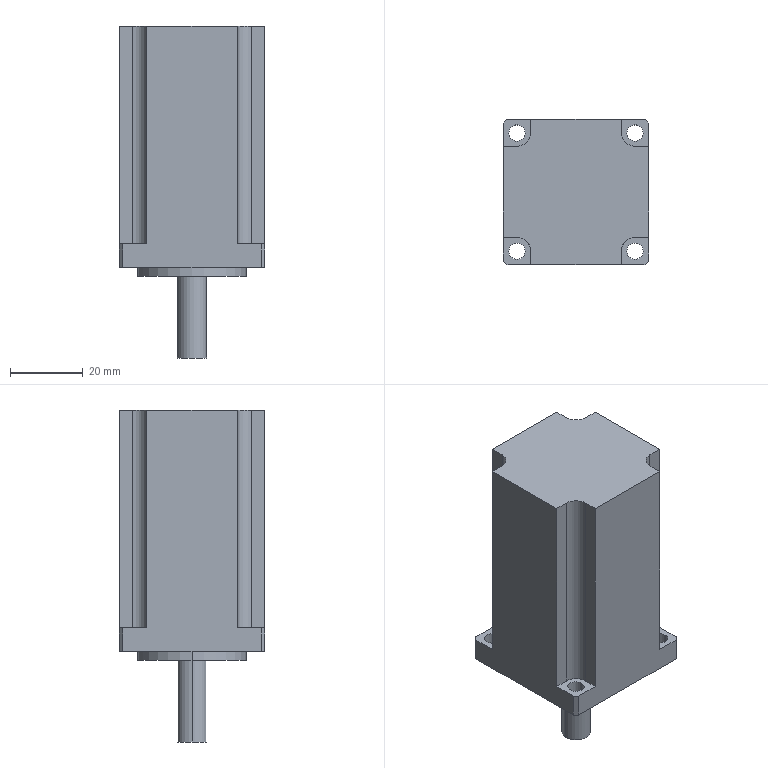Part | Creo | features CURVE 4, DATUM PLANE 3, PROTRUSION 3, CHAMFER 1, COORDINATE SYSTEM 1, CUT 1 | 1 solid | 40 faces | box 40 x 40 x 91.4 mm | volume 96010 mm3 | plane 24 | cylinder 16 | commonest cylinder face diameters 4.5 x8 7.48 x4 8 x2 30 x2
STEP:
#1=CARTESIAN_POINT('',(0.,0.,0.));
#2=DIRECTION('',(0.,0.,1.));
#3=DIRECTION('',(1.,0.,0.));
#4=AXIS2_PLACEMENT_3D('',#1,#2,#3);
#5=CARTESIAN_POINT('',(19.,20.,0.));
#6=VERTEX_POINT('',#5);
#7=CARTESIAN_POINT('',(20.,19.,0.));
#8=VERTEX_POINT('',#7);
#9=CARTESIAN_POINT('',(19.,20.,0.));
#10=DIRECTION('',(0.7071,-0.7071,0.));
#11=VECTOR('',#10,1.414);
#12=LINE('',#9,#11);
#13=EDGE_CURVE('',#6,#8,#12,.T.);
#14=ORIENTED_EDGE('',*,*,#13,.F.);
#15=CARTESIAN_POINT('',(-19.,20.,0.));
#16=VERTEX_POINT('',#15);
#17=CARTESIAN_POINT('',(19.,20.,0.));
#18=DIRECTION('',(-1.,0.,0.));
#19=VECTOR('',#18,38.);
#20=LINE('',#17,#19);
#21=EDGE_CURVE('',#6,#16,#20,.T.);
#22=ORIENTED_EDGE('',*,*,#21,.T.);
#23=CARTESIAN_POINT('',(-20.,19.,0.));
#24=VERTEX_POINT('',#23);
#25=CARTESIAN_POINT('',(-20.,19.,0.));
#26=DIRECTION('',(0.7071,0.7071,0.));
#27=VECTOR('',#26,1.414);
#28=LINE('',#25,#27);
#29=EDGE_CURVE('',#24,#16,#28,.T.);
#30=ORIENTED_EDGE('',*,*,#29,.F.);
#31=CARTESIAN_POINT('',(-20.,-19.,0.));
#32=VERTEX_POINT('',#31);
#33=CARTESIAN_POINT('',(-20.,19.,0.));
#34=DIRECTION('',(0.,-1.,0.));
#35=VECTOR('',#34,38.);
#36=LINE('',#33,#35);
#37=EDGE_CURVE('',#24,#32,#36,.T.);
#38=ORIENTED_EDGE('',*,*,#37,.T.);
#39=CARTESIAN_POINT('',(-19.,-20.,0.));
#40=VERTEX_POINT('',#39);
#41=CARTESIAN_POINT('',(-19.,-20.,0.));
#42=DIRECTION('',(-0.7071,0.7071,0.));
#43=VECTOR('',#42,1.414);
#44=LINE('',#41,#43);
#45=EDGE_CURVE('',#40,#32,#44,.T.);
#46=ORIENTED_EDGE('',*,*,#45,.F.);
#47=CARTESIAN_POINT('',(19.,-20.,0.));
#48=VERTEX_POINT('',#47);
#49=CARTESIAN_POINT('',(-19.,-20.,0.));
#50=DIRECTION('',(1.,0.,0.));
#51=VECTOR('',#50,38.);
#52=LINE('',#49,#51);
#53=EDGE_CURVE('',#40,#48,#52,.T.);
#54=ORIENTED_EDGE('',*,*,#53,.T.);
#55=CARTESIAN_POINT('',(20.,-19.,0.));
#56=VERTEX_POINT('',#55);
#57=CARTESIAN_POINT('',(20.,-19.,0.));
#58=DIRECTION('',(-0.7071,-0.7071,0.));
#59=VECTOR('',#58,1.414);
#60=LINE('',#57,#59);
#61=EDGE_CURVE('',#56,#48,#60,.T.);
#62=ORIENTED_EDGE('',*,*,#61,.F.);
#63=CARTESIAN_POINT('',(20.,-19.,0.));
#64=DIRECTION('',(0.,1.,0.));
#65=VECTOR('',#64,38.);
#66=LINE('',#63,#65);
#67=EDGE_CURVE('',#56,#8,#66,.T.);
#68=ORIENTED_EDGE('',*,*,#67,.T.);
#69=EDGE_LOOP('',(#14,#22,#30,#38,#46,#54,#62,#68));
#70=FACE_OUTER_BOUND('',#69,.F.);
#71=CARTESIAN_POINT('',(-14.01,16.26,0.));
#72=VERTEX_POINT('',#71);
#73=CARTESIAN_POINT('',(-18.51,16.26,0.));
#74=VERTEX_POINT('',#73);
#75=CARTESIAN_POINT('',(-16.26,16.26,0.));
#76=DIRECTION('',(0.,0.,-1.));
#77=DIRECTION('',(1.,0.,0.));
#78=AXIS2_PLACEMENT_3D('',#75,#76,#77);
#79=CIRCLE('',#78,2.25);
#80=EDGE_CURVE('',#72,#74,#79,.T.);
#81=ORIENTED_EDGE('',*,*,#80,.T.);
#82=CARTESIAN_POINT('',(-16.26,16.26,0.));
#83=DIRECTION('',(0.,0.,-1.));
#84=DIRECTION('',(-1.,0.,0.));
#85=AXIS2_PLACEMENT_3D('',#82,#83,#84);
#86=CIRCLE('',#85,2.25);
#87=EDGE_CURVE('',#74,#72,#86,.T.);
#88=ORIENTED_EDGE('',*,*,#87,.T.);
#89=EDGE_LOOP('',(#81,#88));
#90=FACE_BOUND('',#89,.F.);
#91=CARTESIAN_POINT('',(-14.01,-16.26,0.));
#92=VERTEX_POINT('',#91);
#93=CARTESIAN_POINT('',(-18.51,-16.26,0.));
#94=VERTEX_POINT('',#93);
#95=CARTESIAN_POINT('',(-16.26,-16.26,0.));
#96=DIRECTION('',(0.,0.,-1.));
#97=DIRECTION('',(1.,0.,0.));
#98=AXIS2_PLACEMENT_3D('',#95,#96,#97);
#99=CIRCLE('',#98,2.25);
#100=EDGE_CURVE('',#92,#94,#99,.T.);
#101=ORIENTED_EDGE('',*,*,#100,.T.);
#102=CARTESIAN_POINT('',(-16.26,-16.26,0.));
#103=DIRECTION('',(0.,0.,-1.));
#104=DIRECTION('',(-1.,0.,0.));
#105=AXIS2_PLACEMENT_3D('',#102,#103,#104);
#106=CIRCLE('',#105,2.25);
#107=EDGE_CURVE('',#94,#92,#106,.T.);
#108=ORIENTED_EDGE('',*,*,#107,.T.);
#109=EDGE_LOOP('',(#101,#108));
#110=FACE_BOUND('',#109,.F.);
#111=CARTESIAN_POINT('',(18.51,-16.26,0.));
#112=VERTEX_POINT('',#111);
#113=CARTESIAN_POINT('',(14.01,-16.26,0.));
#114=VERTEX_POINT('',#113);
#115=CARTESIAN_POINT('',(16.26,-16.26,0.));
#116=DIRECTION('',(0.,0.,-1.));
#117=DIRECTION('',(1.,0.,0.));
#118=AXIS2_PLACEMENT_3D('',#115,#116,#117);
#119=CIRCLE('',#118,2.25);
#120=EDGE_CURVE('',#112,#114,#119,.T.);
#121=ORIENTED_EDGE('',*,*,#120,.T.);
#122=CARTESIAN_POINT('',(16.26,-16.26,0.));
#123=DIRECTION('',(0.,0.,-1.));
#124=DIRECTION('',(-1.,0.,0.));
#125=AXIS2_PLACEMENT_3D('',#122,#123,#124);
#126=CIRCLE('',#125,2.25);
#127=EDGE_CURVE('',#114,#112,#126,.T.);
#128=ORIENTED_EDGE('',*,*,#127,.T.);
#129=EDGE_LOOP('',(#121,#128));
#130=FACE_BOUND('',#129,.F.);
#131=CARTESIAN_POINT('',(18.51,16.26,0.));
#132=VERTEX_POINT('',#131);
#133=CARTESIAN_POINT('',(14.01,16.26,0.));
#134=VERTEX_POINT('',#133);
#135=CARTESIAN_POINT('',(16.26,16.26,0.));
#136=DIRECTION('',(0.,0.,-1.));
#137=DIRECTION('',(1.,0.,0.));
#138=AXIS2_PLACEMENT_3D('',#135,#136,#137);
#139=CIRCLE('',#138,2.25);
#140=EDGE_CURVE('',#132,#134,#139,.T.);
#141=ORIENTED_EDGE('',*,*,#140,.T.);
#142=CARTESIAN_POINT('',(16.26,16.26,0.));
#143=DIRECTION('',(0.,0.,-1.));
#144=DIRECTION('',(-1.,0.,0.));
#145=AXIS2_PLACEMENT_3D('',#142,#143,#144);
#146=CIRCLE('',#145,2.25);
#147=EDGE_CURVE('',#134,#132,#146,.T.);
#148=ORIENTED_EDGE('',*,*,#147,.T.);
#149=EDGE_LOOP('',(#141,#148));
#150=FACE_BOUND('',#149,.F.);
#151=CARTESIAN_POINT('',(-15.,0.,0.));
#152=VERTEX_POINT('',#151);
#153=CARTESIAN_POINT('',(15.,0.,0.));
#154=VERTEX_POINT('',#153);
#155=CARTESIAN_POINT('',(0.,0.,0.));
#156=DIRECTION('',(0.,0.,-1.));
#157=DIRECTION('',(-1.,0.,0.));
#158=AXIS2_PLACEMENT_3D('',#155,#156,#157);
#159=CIRCLE('',#158,15.);
#160=EDGE_CURVE('',#152,#154,#159,.T.);
#161=ORIENTED_EDGE('',*,*,#160,.T.);
#162=CARTESIAN_POINT('',(0.,0.,0.));
#163=DIRECTION('',(0.,0.,-1.));
#164=DIRECTION('',(1.,0.,0.));
#165=AXIS2_PLACEMENT_3D('',#162,#163,#164);
#166=CIRCLE('',#165,15.);
#167=EDGE_CURVE('',#154,#152,#166,.T.);
#168=ORIENTED_EDGE('',*,*,#167,.T.);
#169=EDGE_LOOP('',(#161,#168));
#170=FACE_BOUND('',#169,.F.);
#171=CARTESIAN_POINT('',(0.,0.,0.));
#172=DIRECTION('',(0.,0.,1.));
#173=DIRECTION('',(1.,0.,0.));
#174=AXIS2_PLACEMENT_3D('',#171,#172,#173);
#175=PLANE('',#174);
#176=ADVANCED_FACE('',(#70,#90,#110,#130,#150,#170),#175,.F.);
#177=CARTESIAN_POINT('',(14.01,16.26,6.4));
#178=VERTEX_POINT('',#177);
#179=CARTESIAN_POINT('',(18.51,16.26,6.4));
#180=VERTEX_POINT('',#179);
#181=CARTESIAN_POINT('',(16.26,16.26,6.4));
#182=DIRECTION('',(0.,0.,1.));
#183=DIRECTION('',(-1.,0.,0.));
#184=AXIS2_PLACEMENT_3D('',#181,#182,#183);
#185=CIRCLE('',#184,2.25);
#186=EDGE_CURVE('',#178,#180,#185,.T.);
#187=ORIENTED_EDGE('',*,*,#186,.F.);
#188=CARTESIAN_POINT('',(14.01,16.26,0.));
#189=DIRECTION('',(0.,0.,1.));
#190=VECTOR('',#189,6.4);
#191=LINE('',#188,#190);
#192=EDGE_CURVE('',#134,#178,#191,.T.);
#193=ORIENTED_EDGE('',*,*,#192,.F.);
#194=ORIENTED_EDGE('',*,*,#140,.F.);
#195=CARTESIAN_POINT('',(18.51,16.26,0.));
#196=DIRECTION('',(0.,0.,1.));
#197=VECTOR('',#196,6.4);
#198=LINE('',#195,#197);
#199=EDGE_CURVE('',#132,#180,#198,.T.);
#200=ORIENTED_EDGE('',*,*,#199,.T.);
#201=EDGE_LOOP('',(#187,#193,#194,#200));
#202=FACE_OUTER_BOUND('',#201,.F.);
#203=CARTESIAN_POINT('',(16.26,16.26,0.));
#204=DIRECTION('',(0.,0.,1.));
#205=DIRECTION('',(1.,0.,0.));
#206=AXIS2_PLACEMENT_3D('',#203,#204,#205);
#207=CYLINDRICAL_SURFACE('',#206,2.25);
#208=ADVANCED_FACE('',(#202),#207,.F.);
#209=CARTESIAN_POINT('',(20.,19.,6.4));
#210=VERTEX_POINT('',#209);
#211=CARTESIAN_POINT('',(19.,20.,6.4));
#212=VERTEX_POINT('',#211);
#213=CARTESIAN_POINT('',(20.,19.,6.4));
#214=DIRECTION('',(-0.7071,0.7071,0.));
#215=VECTOR('',#214,1.414);
#216=LINE('',#213,#215);
#217=EDGE_CURVE('',#210,#212,#216,.T.);
#218=ORIENTED_EDGE('',*,*,#217,.F.);
#219=CARTESIAN_POINT('',(20.,12.52,6.4));
#220=VERTEX_POINT('',#219);
#221=CARTESIAN_POINT('',(20.,12.52,6.4));
#222=DIRECTION('',(0.,1.,0.));
#223=VECTOR('',#222,6.48);
#224=LINE('',#221,#223);
#225=EDGE_CURVE('',#220,#210,#224,.T.);
#226=ORIENTED_EDGE('',*,*,#225,.F.);
#227=CARTESIAN_POINT('',(16.26,12.52,6.4));
#228=VERTEX_POINT('',#227);
#229=CARTESIAN_POINT('',(16.26,12.52,6.4));
#230=DIRECTION('',(1.,0.,0.));
#231=VECTOR('',#230,3.74);
#232=LINE('',#229,#231);
#233=EDGE_CURVE('',#228,#220,#232,.T.);
#234=ORIENTED_EDGE('',*,*,#233,.F.);
#235=CARTESIAN_POINT('',(12.52,16.26,6.4));
#236=VERTEX_POINT('',#235);
#237=CARTESIAN_POINT('',(16.26,16.26,6.4));
#238=DIRECTION('',(0.,0.,1.));
#239=DIRECTION('',(-1.,0.,0.));
#240=AXIS2_PLACEMENT_3D('',#237,#238,#239);
#241=CIRCLE('',#240,3.74);
#242=EDGE_CURVE('',#236,#228,#241,.T.);
#243=ORIENTED_EDGE('',*,*,#242,.F.);
#244=CARTESIAN_POINT('',(12.52,20.,6.4));
#245=VERTEX_POINT('',#244);
#246=CARTESIAN_POINT('',(12.52,20.,6.4));
#247=DIRECTION('',(0.,-1.,0.));
#248=VECTOR('',#247,3.74);
#249=LINE('',#246,#248);
#250=EDGE_CURVE('',#245,#236,#249,.T.);
#251=ORIENTED_EDGE('',*,*,#250,.F.);
#252=CARTESIAN_POINT('',(19.,20.,6.4));
#253=DIRECTION('',(-1.,0.,0.));
#254=VECTOR('',#253,6.48);
#255=LINE('',#252,#254);
#256=EDGE_CURVE('',#212,#245,#255,.T.);
#257=ORIENTED_EDGE('',*,*,#256,.F.);
#258=EDGE_LOOP('',(#218,#226,#234,#243,#251,#257));
#259=FACE_OUTER_BOUND('',#258,.F.);
#260=ORIENTED_EDGE('',*,*,#186,.T.);
#261=CARTESIAN_POINT('',(16.26,16.26,6.4));
#262=DIRECTION('',(0.,0.,1.));
#263=DIRECTION('',(1.,0.,0.));
#264=AXIS2_PLACEMENT_3D('',#261,#262,#263);
#265=CIRCLE('',#264,2.25);
#266=EDGE_CURVE('',#180,#178,#265,.T.);
#267=ORIENTED_EDGE('',*,*,#266,.T.);
#268=EDGE_LOOP('',(#260,#267));
#269=FACE_BOUND('',#268,.F.);
#270=CARTESIAN_POINT('',(0.,0.,6.4));
#271=DIRECTION('',(0.,0.,1.));
#272=DIRECTION('',(1.,0.,0.));
#273=AXIS2_PLACEMENT_3D('',#270,#271,#272);
#274=PLANE('',#273);
#275=ADVANCED_FACE('',(#259,#269),#274,.T.);
#276=CARTESIAN_POINT('',(19.,-20.,6.4));
#277=VERTEX_POINT('',#276);
#278=CARTESIAN_POINT('',(20.,-19.,6.4));
#279=VERTEX_POINT('',#278);
#280=CARTESIAN_POINT('',(19.,-20.,6.4));
#281=DIRECTION('',(0.7071,0.7071,0.));
#282=VECTOR('',#281,1.414);
#283=LINE('',#280,#282);
#284=EDGE_CURVE('',#277,#279,#283,.T.);
#285=ORIENTED_EDGE('',*,*,#284,.F.);
#286=CARTESIAN_POINT('',(12.52,-20.,6.4));
#287=VERTEX_POINT('',#286);
#288=CARTESIAN_POINT('',(12.52,-20.,6.4));
#289=DIRECTION('',(1.,0.,0.));
#290=VECTOR('',#289,6.48);
#291=LINE('',#288,#290);
#292=EDGE_CURVE('',#287,#277,#291,.T.);
#293=ORIENTED_EDGE('',*,*,#292,.F.);
#294=CARTESIAN_POINT('',(12.52,-16.26,6.4));
#295=VERTEX_POINT('',#294);
#296=CARTESIAN_POINT('',(12.52,-16.26,6.4));
#297=DIRECTION('',(0.,-1.,0.));
#298=VECTOR('',#297,3.74);
#299=LINE('',#296,#298);
#300=EDGE_CURVE('',#295,#287,#299,.T.);
#301=ORIENTED_EDGE('',*,*,#300,.F.);
#302=CARTESIAN_POINT('',(16.26,-12.52,6.4));
#303=VERTEX_POINT('',#302);
#304=CARTESIAN_POINT('',(16.26,-16.26,6.4));
#305=DIRECTION('',(0.,0.,1.));
#306=DIRECTION('',(0.,1.,0.));
#307=AXIS2_PLACEMENT_3D('',#304,#305,#306);
#308=CIRCLE('',#307,3.74);
#309=EDGE_CURVE('',#303,#295,#308,.T.);
#310=ORIENTED_EDGE('',*,*,#309,.F.);
#311=CARTESIAN_POINT('',(20.,-12.52,6.4));
#312=VERTEX_POINT('',#311);
#313=CARTESIAN_POINT('',(20.,-12.52,6.4));
#314=DIRECTION('',(-1.,0.,0.));
#315=VECTOR('',#314,3.74);
#316=LINE('',#313,#315);
#317=EDGE_CURVE('',#312,#303,#316,.T.);
#318=ORIENTED_EDGE('',*,*,#317,.F.);
#319=CARTESIAN_POINT('',(20.,-19.,6.4));
#320=DIRECTION('',(0.,1.,0.));
#321=VECTOR('',#320,6.48);
#322=LINE('',#319,#321);
#323=EDGE_CURVE('',#279,#312,#322,.T.);
#324=ORIENTED_EDGE('',*,*,#323,.F.);
#325=EDGE_LOOP('',(#285,#293,#301,#310,#318,#324));
#326=FACE_OUTER_BOUND('',#325,.F.);
#327=CARTESIAN_POINT('',(14.01,-16.26,6.4));
#328=VERTEX_POINT('',#327);
#329=CARTESIAN_POINT('',(18.51,-16.26,6.4));
#330=VERTEX_POINT('',#329);
#331=CARTESIAN_POINT('',(16.26,-16.26,6.4));
#332=DIRECTION('',(0.,0.,1.));
#333=DIRECTION('',(-1.,0.,0.));
#334=AXIS2_PLACEMENT_3D('',#331,#332,#333);
#335=CIRCLE('',#334,2.25);
#336=EDGE_CURVE('',#328,#330,#335,.T.);
#337=ORIENTED_EDGE('',*,*,#336,.T.);
#338=CARTESIAN_POINT('',(16.26,-16.26,6.4));
#339=DIRECTION('',(0.,0.,1.));
#340=DIRECTION('',(1.,0.,0.));
#341=AXIS2_PLACEMENT_3D('',#338,#339,#340);
#342=CIRCLE('',#341,2.25);
#343=EDGE_CURVE('',#330,#328,#342,.T.);
#344=ORIENTED_EDGE('',*,*,#343,.T.);
#345=EDGE_LOOP('',(#337,#344));
#346=FACE_BOUND('',#345,.F.);
#347=CARTESIAN_POINT('',(0.,0.,6.4));
#348=DIRECTION('',(0.,0.,1.));
#349=DIRECTION('',(1.,0.,0.));
#350=AXIS2_PLACEMENT_3D('',#347,#348,#349);
#351=PLANE('',#350);
#352=ADVANCED_FACE('',(#326,#346),#351,.T.);
#353=CARTESIAN_POINT('',(-20.,-19.,6.4));
#354=VERTEX_POINT('',#353);
#355=CARTESIAN_POINT('',(-19.,-20.,6.4));
#356=VERTEX_POINT('',#355);
#357=CARTESIAN_POINT('',(-20.,-19.,6.4));
#358=DIRECTION('',(0.7071,-0.7071,0.));
#359=VECTOR('',#358,1.414);
#360=LINE('',#357,#359);
#361=EDGE_CURVE('',#354,#356,#360,.T.);
#362=ORIENTED_EDGE('',*,*,#361,.F.);
#363=CARTESIAN_POINT('',(-20.,-12.52,6.4));
#364=VERTEX_POINT('',#363);
#365=CARTESIAN_POINT('',(-20.,-12.52,6.4));
#366=DIRECTION('',(0.,-1.,0.));
#367=VECTOR('',#366,6.48);
#368=LINE('',#365,#367);
#369=EDGE_CURVE('',#364,#354,#368,.T.);
#370=ORIENTED_EDGE('',*,*,#369,.F.);
#371=CARTESIAN_POINT('',(-16.26,-12.52,6.4));
#372=VERTEX_POINT('',#371);
#373=CARTESIAN_POINT('',(-16.26,-12.52,6.4));
#374=DIRECTION('',(-1.,0.,0.));
#375=VECTOR('',#374,3.74);
#376=LINE('',#373,#375);
#377=EDGE_CURVE('',#372,#364,#376,.T.);
#378=ORIENTED_EDGE('',*,*,#377,.F.);
#379=CARTESIAN_POINT('',(-12.52,-16.26,6.4));
#380=VERTEX_POINT('',#379);
#381=CARTESIAN_POINT('',(-16.26,-16.26,6.4));
#382=DIRECTION('',(0.,0.,1.));
#383=DIRECTION('',(1.,0.,0.));
#384=AXIS2_PLACEMENT_3D('',#381,#382,#383);
#385=CIRCLE('',#384,3.74);
#386=EDGE_CURVE('',#380,#372,#385,.T.);
#387=ORIENTED_EDGE('',*,*,#386,.F.);
#388=CARTESIAN_POINT('',(-12.52,-20.,6.4));
#389=VERTEX_POINT('',#388);
#390=CARTESIAN_POINT('',(-12.52,-20.,6.4));
#391=DIRECTION('',(0.,1.,0.));
#392=VECTOR('',#391,3.74);
#393=LINE('',#390,#392);
#394=EDGE_CURVE('',#389,#380,#393,.T.);
#395=ORIENTED_EDGE('',*,*,#394,.F.);
#396=CARTESIAN_POINT('',(-19.,-20.,6.4));
#397=DIRECTION('',(1.,0.,0.));
#398=VECTOR('',#397,6.48);
#399=LINE('',#396,#398);
#400=EDGE_CURVE('',#356,#389,#399,.T.);
#401=ORIENTED_EDGE('',*,*,#400,.F.);
#402=EDGE_LOOP('',(#362,#370,#378,#387,#395,#401));
#403=FACE_OUTER_BOUND('',#402,.F.);
#404=CARTESIAN_POINT('',(-18.51,-16.26,6.4));
#405=VERTEX_POINT('',#404);
#406=CARTESIAN_POINT('',(-14.01,-16.26,6.4));
#407=VERTEX_POINT('',#406);
#408=CARTESIAN_POINT('',(-16.26,-16.26,6.4));
#409=DIRECTION('',(0.,0.,1.));
#410=DIRECTION('',(-1.,0.,0.));
#411=AXIS2_PLACEMENT_3D('',#408,#409,#410);
#412=CIRCLE('',#411,2.25);
#413=EDGE_CURVE('',#405,#407,#412,.T.);
#414=ORIENTED_EDGE('',*,*,#413,.T.);
#415=CARTESIAN_POINT('',(-16.26,-16.26,6.4));
#416=DIRECTION('',(0.,0.,1.));
#417=DIRECTION('',(1.,0.,0.));
#418=AXIS2_PLACEMENT_3D('',#415,#416,#417);
#419=CIRCLE('',#418,2.25);
#420=EDGE_CURVE('',#407,#405,#419,.T.);
#421=ORIENTED_EDGE('',*,*,#420,.T.);
#422=EDGE_LOOP('',(#414,#421));
#423=FACE_BOUND('',#422,.F.);
#424=CARTESIAN_POINT('',(0.,0.,6.4));
#425=DIRECTION('',(0.,0.,1.));
#426=DIRECTION('',(1.,0.,0.));
#427=AXIS2_PLACEMENT_3D('',#424,#425,#426);
#428=PLANE('',#427);
#429=ADVANCED_FACE('',(#403,#423),#428,.T.);
#430=CARTESIAN_POINT('',(-19.,20.,6.4));
#431=VERTEX_POINT('',#430);
#432=CARTESIAN_POINT('',(-20.,19.,6.4));
#433=VERTEX_POINT('',#432);
#434=CARTESIAN_POINT('',(-19.,20.,6.4));
#435=DIRECTION('',(-0.7071,-0.7071,0.));
#436=VECTOR('',#435,1.414);
#437=LINE('',#434,#436);
#438=EDGE_CURVE('',#431,#433,#437,.T.);
#439=ORIENTED_EDGE('',*,*,#438,.F.);
#440=CARTESIAN_POINT('',(-12.52,20.,6.4));
#441=VERTEX_POINT('',#440);
#442=CARTESIAN_POINT('',(-12.52,20.,6.4));
#443=DIRECTION('',(-1.,0.,0.));
#444=VECTOR('',#443,6.48);
#445=LINE('',#442,#444);
#446=EDGE_CURVE('',#441,#431,#445,.T.);
#447=ORIENTED_EDGE('',*,*,#446,.F.);
#448=CARTESIAN_POINT('',(-12.52,16.26,6.4));
#449=VERTEX_POINT('',#448);
#450=CARTESIAN_POINT('',(-12.52,16.26,6.4));
#451=DIRECTION('',(0.,1.,0.));
#452=VECTOR('',#451,3.74);
#453=LINE('',#450,#452);
#454=EDGE_CURVE('',#449,#441,#453,.T.);
#455=ORIENTED_EDGE('',*,*,#454,.F.);
#456=CARTESIAN_POINT('',(-16.26,12.52,6.4));
#457=VERTEX_POINT('',#456);
#458=CARTESIAN_POINT('',(-16.26,16.26,6.4));
#459=DIRECTION('',(0.,0.,1.));
#460=DIRECTION('',(0.,-1.,0.));
#461=AXIS2_PLACEMENT_3D('',#458,#459,#460);
#462=CIRCLE('',#461,3.74);
#463=EDGE_CURVE('',#457,#449,#462,.T.);
#464=ORIENTED_EDGE('',*,*,#463,.F.);
#465=CARTESIAN_POINT('',(-20.,12.52,6.4));
#466=VERTEX_POINT('',#465);
#467=CARTESIAN_POINT('',(-20.,12.52,6.4));
#468=DIRECTION('',(1.,0.,0.));
#469=VECTOR('',#468,3.74);
#470=LINE('',#467,#469);
#471=EDGE_CURVE('',#466,#457,#470,.T.);
#472=ORIENTED_EDGE('',*,*,#471,.F.);
#473=CARTESIAN_POINT('',(-20.,19.,6.4));
#474=DIRECTION('',(0.,-1.,0.));
#475=VECTOR('',#474,6.48);
#476=LINE('',#473,#475);
#477=EDGE_CURVE('',#433,#466,#476,.T.);
#478=ORIENTED_EDGE('',*,*,#477,.F.);
#479=EDGE_LOOP('',(#439,#447,#455,#464,#472,#478));
#480=FACE_OUTER_BOUND('',#479,.F.);
#481=CARTESIAN_POINT('',(-18.51,16.26,6.4));
#482=VERTEX_POINT('',#481);
#483=CARTESIAN_POINT('',(-14.01,16.26,6.4));
#484=VERTEX_POINT('',#483);
#485=CARTESIAN_POINT('',(-16.26,16.26,6.4));
#486=DIRECTION('',(0.,0.,1.));
#487=DIRECTION('',(-1.,0.,0.));
#488=AXIS2_PLACEMENT_3D('',#485,#486,#487);
#489=CIRCLE('',#488,2.25);
#490=EDGE_CURVE('',#482,#484,#489,.T.);
#491=ORIENTED_EDGE('',*,*,#490,.T.);
#492=CARTESIAN_POINT('',(-16.26,16.26,6.4));
#493=DIRECTION('',(0.,0.,1.));
#494=DIRECTION('',(1.,0.,0.));
#495=AXIS2_PLACEMENT_3D('',#492,#493,#494);
#496=CIRCLE('',#495,2.25);
#497=EDGE_CURVE('',#484,#482,#496,.T.);
#498=ORIENTED_EDGE('',*,*,#497,.T.);
#499=EDGE_LOOP('',(#491,#498));
#500=FACE_BOUND('',#499,.F.);
#501=CARTESIAN_POINT('',(0.,0.,6.4));
#502=DIRECTION('',(0.,0.,1.));
#503=DIRECTION('',(1.,0.,0.));
#504=AXIS2_PLACEMENT_3D('',#501,#502,#503);
#505=PLANE('',#504);
#506=ADVANCED_FACE('',(#480,#500),#505,.T.);
#507=ORIENTED_EDGE('',*,*,#336,.F.);
#508=CARTESIAN_POINT('',(14.01,-16.26,0.));
#509=DIRECTION('',(0.,0.,1.));
#510=VECTOR('',#509,6.4);
#511=LINE('',#508,#510);
#512=EDGE_CURVE('',#114,#328,#511,.T.);
#513=ORIENTED_EDGE('',*,*,#512,.F.);
#514=ORIENTED_EDGE('',*,*,#120,.F.);
#515=CARTESIAN_POINT('',(18.51,-16.26,0.));
#516=DIRECTION('',(0.,0.,1.));
#517=VECTOR('',#516,6.4);
#518=LINE('',#515,#517);
#519=EDGE_CURVE('',#112,#330,#518,.T.);
#520=ORIENTED_EDGE('',*,*,#519,.T.);
#521=EDGE_LOOP('',(#507,#513,#514,#520));
#522=FACE_OUTER_BOUND('',#521,.F.);
#523=CARTESIAN_POINT('',(16.26,-16.26,0.));
#524=DIRECTION('',(0.,0.,1.));
#525=DIRECTION('',(1.,0.,0.));
#526=AXIS2_PLACEMENT_3D('',#523,#524,#525);
#527=CYLINDRICAL_SURFACE('',#526,2.25);
#528=ADVANCED_FACE('',(#522),#527,.F.);
#529=ORIENTED_EDGE('',*,*,#343,.F.);
#530=ORIENTED_EDGE('',*,*,#519,.F.);
#531=ORIENTED_EDGE('',*,*,#127,.F.);
#532=ORIENTED_EDGE('',*,*,#512,.T.);
#533=EDGE_LOOP('',(#529,#530,#531,#532));
#534=FACE_OUTER_BOUND('',#533,.F.);
#535=CARTESIAN_POINT('',(16.26,-16.26,0.));
#536=DIRECTION('',(0.,0.,1.));
#537=DIRECTION('',(1.,0.,0.));
#538=AXIS2_PLACEMENT_3D('',#535,#536,#537);
#539=CYLINDRICAL_SURFACE('',#538,2.25);
#540=ADVANCED_FACE('',(#534),#539,.F.);
#541=ORIENTED_EDGE('',*,*,#266,.F.);
#542=ORIENTED_EDGE('',*,*,#199,.F.);
#543=ORIENTED_EDGE('',*,*,#147,.F.);
#544=ORIENTED_EDGE('',*,*,#192,.T.);
#545=EDGE_LOOP('',(#541,#542,#543,#544));
#546=FACE_OUTER_BOUND('',#545,.F.);
#547=CARTESIAN_POINT('',(16.26,16.26,0.));
#548=DIRECTION('',(0.,0.,1.));
#549=DIRECTION('',(1.,0.,0.));
#550=AXIS2_PLACEMENT_3D('',#547,#548,#549);
#551=CYLINDRICAL_SURFACE('',#550,2.25);
#552=ADVANCED_FACE('',(#546),#551,.F.);
#553=ORIENTED_EDGE('',*,*,#490,.F.);
#554=CARTESIAN_POINT('',(-18.51,16.26,0.));
#555=DIRECTION('',(0.,0.,1.));
#556=VECTOR('',#555,6.4);
#557=LINE('',#554,#556);
#558=EDGE_CURVE('',#74,#482,#557,.T.);
#559=ORIENTED_EDGE('',*,*,#558,.F.);
#560=ORIENTED_EDGE('',*,*,#80,.F.);
#561=CARTESIAN_POINT('',(-14.01,16.26,0.));
#562=DIRECTION('',(0.,0.,1.));
#563=VECTOR('',#562,6.4);
#564=LINE('',#561,#563);
#565=EDGE_CURVE('',#72,#484,#564,.T.);
#566=ORIENTED_EDGE('',*,*,#565,.T.);
#567=EDGE_LOOP('',(#553,#559,#560,#566));
#568=FACE_OUTER_BOUND('',#567,.F.);
#569=CARTESIAN_POINT('',(-16.26,16.26,0.));
#570=DIRECTION('',(0.,0.,1.));
#571=DIRECTION('',(1.,0.,0.));
#572=AXIS2_PLACEMENT_3D('',#569,#570,#571);
#573=CYLINDRICAL_SURFACE('',#572,2.25);
#574=ADVANCED_FACE('',(#568),#573,.F.);
#575=ORIENTED_EDGE('',*,*,#497,.F.);
#576=ORIENTED_EDGE('',*,*,#565,.F.);
#577=ORIENTED_EDGE('',*,*,#87,.F.);
#578=ORIENTED_EDGE('',*,*,#558,.T.);
#579=EDGE_LOOP('',(#575,#576,#577,#578));
#580=FACE_OUTER_BOUND('',#579,.F.);
#581=CARTESIAN_POINT('',(-16.26,16.26,0.));
#582=DIRECTION('',(0.,0.,1.));
#583=DIRECTION('',(1.,0.,0.));
#584=AXIS2_PLACEMENT_3D('',#581,#582,#583);
#585=CYLINDRICAL_SURFACE('',#584,2.25);
#586=ADVANCED_FACE('',(#580),#585,.F.);
#587=ORIENTED_EDGE('',*,*,#413,.F.);
#588=CARTESIAN_POINT('',(-18.51,-16.26,0.));
#589=DIRECTION('',(0.,0.,1.));
#590=VECTOR('',#589,6.4);
#591=LINE('',#588,#590);
#592=EDGE_CURVE('',#94,#405,#591,.T.);
#593=ORIENTED_EDGE('',*,*,#592,.F.);
#594=ORIENTED_EDGE('',*,*,#100,.F.);
#595=CARTESIAN_POINT('',(-14.01,-16.26,0.));
#596=DIRECTION('',(0.,0.,1.));
#597=VECTOR('',#596,6.4);
#598=LINE('',#595,#597);
#599=EDGE_CURVE('',#92,#407,#598,.T.);
#600=ORIENTED_EDGE('',*,*,#599,.T.);
#601=EDGE_LOOP('',(#587,#593,#594,#600));
#602=FACE_OUTER_BOUND('',#601,.F.);
#603=CARTESIAN_POINT('',(-16.26,-16.26,0.));
#604=DIRECTION('',(0.,0.,1.));
#605=DIRECTION('',(1.,0.,0.));
#606=AXIS2_PLACEMENT_3D('',#603,#604,#605);
#607=CYLINDRICAL_SURFACE('',#606,2.25);
#608=ADVANCED_FACE('',(#602),#607,.F.);
#609=ORIENTED_EDGE('',*,*,#420,.F.);
#610=ORIENTED_EDGE('',*,*,#599,.F.);
#611=ORIENTED_EDGE('',*,*,#107,.F.);
#612=ORIENTED_EDGE('',*,*,#592,.T.);
#613=EDGE_LOOP('',(#609,#610,#611,#612));
#614=FACE_OUTER_BOUND('',#613,.F.);
#615=CARTESIAN_POINT('',(-16.26,-16.26,0.));
#616=DIRECTION('',(0.,0.,1.));
#617=DIRECTION('',(1.,0.,0.));
#618=AXIS2_PLACEMENT_3D('',#615,#616,#617);
#619=CYLINDRICAL_SURFACE('',#618,2.25);
#620=ADVANCED_FACE('',(#614),#619,.F.);
#621=ORIENTED_EDGE('',*,*,#13,.T.);
#622=CARTESIAN_POINT('',(20.,19.,6.4));
#623=DIRECTION('',(0.,0.,-1.));
#624=VECTOR('',#623,6.4);
#625=LINE('',#622,#624);
#626=EDGE_CURVE('',#210,#8,#625,.T.);
#627=ORIENTED_EDGE('',*,*,#626,.F.);
#628=ORIENTED_EDGE('',*,*,#217,.T.);
#629=CARTESIAN_POINT('',(19.,20.,6.4));
#630=DIRECTION('',(0.,0.,-1.));
#631=VECTOR('',#630,6.4);
#632=LINE('',#629,#631);
#633=EDGE_CURVE('',#212,#6,#632,.T.);
#634=ORIENTED_EDGE('',*,*,#633,.T.);
#635=EDGE_LOOP('',(#621,#627,#628,#634));
#636=FACE_OUTER_BOUND('',#635,.F.);
#637=CARTESIAN_POINT('',(19.5,19.5,3.2));
#638=DIRECTION('',(0.7071,0.7071,0.));
#639=DIRECTION('',(0.7071,-0.7071,0.));
#640=AXIS2_PLACEMENT_3D('',#637,#638,#639);
#641=PLANE('',#640);
#642=ADVANCED_FACE('',(#636),#641,.T.);
#643=ORIENTED_EDGE('',*,*,#626,.T.);
#644=ORIENTED_EDGE('',*,*,#67,.F.);
#645=CARTESIAN_POINT('',(20.,-19.,6.4));
#646=DIRECTION('',(0.,0.,-1.));
#647=VECTOR('',#646,6.4);
#648=LINE('',#645,#647);
#649=EDGE_CURVE('',#279,#56,#648,.T.);
#650=ORIENTED_EDGE('',*,*,#649,.F.);
#651=ORIENTED_EDGE('',*,*,#323,.T.);
#652=CARTESIAN_POINT('',(20.,-12.52,66.4));
#653=VERTEX_POINT('',#652);
#654=CARTESIAN_POINT('',(20.,-12.52,66.4));
#655=DIRECTION('',(0.,0.,-1.));
#656=VECTOR('',#655,60.);
#657=LINE('',#654,#656);
#658=EDGE_CURVE('',#653,#312,#657,.T.);
#659=ORIENTED_EDGE('',*,*,#658,.F.);
#660=CARTESIAN_POINT('',(20.,12.52,66.4));
#661=VERTEX_POINT('',#660);
#662=CARTESIAN_POINT('',(20.,-12.52,66.4));
#663=DIRECTION('',(0.,1.,0.));
#664=VECTOR('',#663,25.04);
#665=LINE('',#662,#664);
#666=EDGE_CURVE('',#653,#661,#665,.T.);
#667=ORIENTED_EDGE('',*,*,#666,.T.);
#668=CARTESIAN_POINT('',(20.,12.52,66.4));
#669=DIRECTION('',(0.,0.,-1.));
#670=VECTOR('',#669,60.);
#671=LINE('',#668,#670);
#672=EDGE_CURVE('',#661,#220,#671,.T.);
#673=ORIENTED_EDGE('',*,*,#672,.T.);
#674=ORIENTED_EDGE('',*,*,#225,.T.);
#675=EDGE_LOOP('',(#643,#644,#650,#651,#659,#667,#673,#674));
#676=FACE_OUTER_BOUND('',#675,.F.);
#677=CARTESIAN_POINT('',(20.,-20.,0.));
#678=DIRECTION('',(1.,0.,0.));
#679=DIRECTION('',(0.,1.,0.));
#680=AXIS2_PLACEMENT_3D('',#677,#678,#679);
#681=PLANE('',#680);
#682=ADVANCED_FACE('',(#676),#681,.T.);
#683=ORIENTED_EDGE('',*,*,#61,.T.);
#684=CARTESIAN_POINT('',(19.,-20.,6.4));
#685=DIRECTION('',(0.,0.,-1.));
#686=VECTOR('',#685,6.4);
#687=LINE('',#684,#686);
#688=EDGE_CURVE('',#277,#48,#687,.T.);
#689=ORIENTED_EDGE('',*,*,#688,.F.);
#690=ORIENTED_EDGE('',*,*,#284,.T.);
#691=ORIENTED_EDGE('',*,*,#649,.T.);
#692=EDGE_LOOP('',(#683,#689,#690,#691));
#693=FACE_OUTER_BOUND('',#692,.F.);
#694=CARTESIAN_POINT('',(19.5,-19.5,3.2));
#695=DIRECTION('',(0.7071,-0.7071,0.));
#696=DIRECTION('',(-0.7071,-0.7071,0.));
#697=AXIS2_PLACEMENT_3D('',#694,#695,#696);
#698=PLANE('',#697);
#699=ADVANCED_FACE('',(#693),#698,.T.);
#700=ORIENTED_EDGE('',*,*,#688,.T.);
#701=ORIENTED_EDGE('',*,*,#53,.F.);
#702=CARTESIAN_POINT('',(-19.,-20.,6.4));
#703=DIRECTION('',(0.,0.,-1.));
#704=VECTOR('',#703,6.4);
#705=LINE('',#702,#704);
#706=EDGE_CURVE('',#356,#40,#705,.T.);
#707=ORIENTED_EDGE('',*,*,#706,.F.);
#708=ORIENTED_EDGE('',*,*,#400,.T.);
#709=CARTESIAN_POINT('',(-12.52,-20.,66.4));
#710=VERTEX_POINT('',#709);
#711=CARTESIAN_POINT('',(-12.52,-20.,66.4));
#712=DIRECTION('',(0.,0.,-1.));
#713=VECTOR('',#712,60.);
#714=LINE('',#711,#713);
#715=EDGE_CURVE('',#710,#389,#714,.T.);
#716=ORIENTED_EDGE('',*,*,#715,.F.);
#717=CARTESIAN_POINT('',(12.52,-20.,66.4));
#718=VERTEX_POINT('',#717);
#719=CARTESIAN_POINT('',(-12.52,-20.,66.4));
#720=DIRECTION('',(1.,0.,0.));
#721=VECTOR('',#720,25.04);
#722=LINE('',#719,#721);
#723=EDGE_CURVE('',#710,#718,#722,.T.);
#724=ORIENTED_EDGE('',*,*,#723,.T.);
#725=CARTESIAN_POINT('',(12.52,-20.,66.4));
#726=DIRECTION('',(0.,0.,-1.));
#727=VECTOR('',#726,60.);
#728=LINE('',#725,#727);
#729=EDGE_CURVE('',#718,#287,#728,.T.);
#730=ORIENTED_EDGE('',*,*,#729,.T.);
#731=ORIENTED_EDGE('',*,*,#292,.T.);
#732=EDGE_LOOP('',(#700,#701,#707,#708,#716,#724,#730,#731));
#733=FACE_OUTER_BOUND('',#732,.F.);
#734=CARTESIAN_POINT('',(-20.,-20.,0.));
#735=DIRECTION('',(0.,-1.,0.));
#736=DIRECTION('',(1.,0.,0.));
#737=AXIS2_PLACEMENT_3D('',#734,#735,#736);
#738=PLANE('',#737);
#739=ADVANCED_FACE('',(#733),#738,.T.);
#740=ORIENTED_EDGE('',*,*,#45,.T.);
#741=CARTESIAN_POINT('',(-20.,-19.,6.4));
#742=DIRECTION('',(0.,0.,-1.));
#743=VECTOR('',#742,6.4);
#744=LINE('',#741,#743);
#745=EDGE_CURVE('',#354,#32,#744,.T.);
#746=ORIENTED_EDGE('',*,*,#745,.F.);
#747=ORIENTED_EDGE('',*,*,#361,.T.);
#748=ORIENTED_EDGE('',*,*,#706,.T.);
#749=EDGE_LOOP('',(#740,#746,#747,#748));
#750=FACE_OUTER_BOUND('',#749,.F.);
#751=CARTESIAN_POINT('',(-19.5,-19.5,3.2));
#752=DIRECTION('',(-0.7071,-0.7071,0.));
#753=DIRECTION('',(-0.7071,0.7071,0.));
#754=AXIS2_PLACEMENT_3D('',#751,#752,#753);
#755=PLANE('',#754);
#756=ADVANCED_FACE('',(#750),#755,.T.);
#757=ORIENTED_EDGE('',*,*,#745,.T.);
#758=ORIENTED_EDGE('',*,*,#37,.F.);
#759=CARTESIAN_POINT('',(-20.,19.,6.4));
#760=DIRECTION('',(0.,0.,-1.));
#761=VECTOR('',#760,6.4);
#762=LINE('',#759,#761);
#763=EDGE_CURVE('',#433,#24,#762,.T.);
#764=ORIENTED_EDGE('',*,*,#763,.F.);
#765=ORIENTED_EDGE('',*,*,#477,.T.);
#766=CARTESIAN_POINT('',(-20.,12.52,66.4));
#767=VERTEX_POINT('',#766);
#768=CARTESIAN_POINT('',(-20.,12.52,66.4));
#769=DIRECTION('',(0.,0.,-1.));
#770=VECTOR('',#769,60.);
#771=LINE('',#768,#770);
#772=EDGE_CURVE('',#767,#466,#771,.T.);
#773=ORIENTED_EDGE('',*,*,#772,.F.);
#774=CARTESIAN_POINT('',(-20.,-12.52,66.4));
#775=VERTEX_POINT('',#774);
#776=CARTESIAN_POINT('',(-20.,12.52,66.4));
#777=DIRECTION('',(0.,-1.,0.));
#778=VECTOR('',#777,25.04);
#779=LINE('',#776,#778);
#780=EDGE_CURVE('',#767,#775,#779,.T.);
#781=ORIENTED_EDGE('',*,*,#780,.T.);
#782=CARTESIAN_POINT('',(-20.,-12.52,66.4));
#783=DIRECTION('',(0.,0.,-1.));
#784=VECTOR('',#783,60.);
#785=LINE('',#782,#784);
#786=EDGE_CURVE('',#775,#364,#785,.T.);
#787=ORIENTED_EDGE('',*,*,#786,.T.);
#788=ORIENTED_EDGE('',*,*,#369,.T.);
#789=EDGE_LOOP('',(#757,#758,#764,#765,#773,#781,#787,#788));
#790=FACE_OUTER_BOUND('',#789,.F.);
#791=CARTESIAN_POINT('',(-20.,20.,0.));
#792=DIRECTION('',(-1.,0.,0.));
#793=DIRECTION('',(0.,-1.,0.));
#794=AXIS2_PLACEMENT_3D('',#791,#792,#793);
#795=PLANE('',#794);
#796=ADVANCED_FACE('',(#790),#795,.T.);
#797=ORIENTED_EDGE('',*,*,#29,.T.);
#798=CARTESIAN_POINT('',(-19.,20.,6.4));
#799=DIRECTION('',(0.,0.,-1.));
#800=VECTOR('',#799,6.4);
#801=LINE('',#798,#800);
#802=EDGE_CURVE('',#431,#16,#801,.T.);
#803=ORIENTED_EDGE('',*,*,#802,.F.);
#804=ORIENTED_EDGE('',*,*,#438,.T.);
#805=ORIENTED_EDGE('',*,*,#763,.T.);
#806=EDGE_LOOP('',(#797,#803,#804,#805));
#807=FACE_OUTER_BOUND('',#806,.F.);
#808=CARTESIAN_POINT('',(-19.5,19.5,3.2));
#809=DIRECTION('',(-0.7071,0.7071,0.));
#810=DIRECTION('',(0.7071,0.7071,0.));
#811=AXIS2_PLACEMENT_3D('',#808,#809,#810);
#812=PLANE('',#811);
#813=ADVANCED_FACE('',(#807),#812,.T.);
#814=ORIENTED_EDGE('',*,*,#633,.F.);
#815=ORIENTED_EDGE('',*,*,#256,.T.);
#816=CARTESIAN_POINT('',(12.52,20.,66.4));
#817=VERTEX_POINT('',#816);
#818=CARTESIAN_POINT('',(12.52,20.,66.4));
#819=DIRECTION('',(0.,0.,-1.));
#820=VECTOR('',#819,60.);
#821=LINE('',#818,#820);
#822=EDGE_CURVE('',#817,#245,#821,.T.);
#823=ORIENTED_EDGE('',*,*,#822,.F.);
#824=CARTESIAN_POINT('',(-12.52,20.,66.4));
#825=VERTEX_POINT('',#824);
#826=CARTESIAN_POINT('',(12.52,20.,66.4));
#827=DIRECTION('',(-1.,0.,0.));
#828=VECTOR('',#827,25.04);
#829=LINE('',#826,#828);
#830=EDGE_CURVE('',#817,#825,#829,.T.);
#831=ORIENTED_EDGE('',*,*,#830,.T.);
#832=CARTESIAN_POINT('',(-12.52,20.,66.4));
#833=DIRECTION('',(0.,0.,-1.));
#834=VECTOR('',#833,60.);
#835=LINE('',#832,#834);
#836=EDGE_CURVE('',#825,#441,#835,.T.);
#837=ORIENTED_EDGE('',*,*,#836,.T.);
#838=ORIENTED_EDGE('',*,*,#446,.T.);
#839=ORIENTED_EDGE('',*,*,#802,.T.);
#840=ORIENTED_EDGE('',*,*,#21,.F.);
#841=EDGE_LOOP('',(#814,#815,#823,#831,#837,#838,#839,#840));
#842=FACE_OUTER_BOUND('',#841,.F.);
#843=CARTESIAN_POINT('',(20.,20.,0.));
#844=DIRECTION('',(0.,1.,0.));
#845=DIRECTION('',(-1.,0.,0.));
#846=AXIS2_PLACEMENT_3D('',#843,#844,#845);
#847=PLANE('',#846);
#848=ADVANCED_FACE('',(#842),#847,.T.);
#849=CARTESIAN_POINT('',(12.52,16.26,66.4));
#850=VERTEX_POINT('',#849);
#851=CARTESIAN_POINT('',(12.52,20.,66.4));
#852=DIRECTION('',(0.,-1.,0.));
#853=VECTOR('',#852,3.74);
#854=LINE('',#851,#853);
#855=EDGE_CURVE('',#817,#850,#854,.T.);
#856=ORIENTED_EDGE('',*,*,#855,.F.);
#857=ORIENTED_EDGE('',*,*,#822,.T.);
#858=ORIENTED_EDGE('',*,*,#250,.T.);
#859=CARTESIAN_POINT('',(12.52,16.26,66.4));
#860=DIRECTION('',(0.,0.,-1.));
#861=VECTOR('',#860,60.);
#862=LINE('',#859,#861);
#863=EDGE_CURVE('',#850,#236,#862,.T.);
#864=ORIENTED_EDGE('',*,*,#863,.F.);
#865=EDGE_LOOP('',(#856,#857,#858,#864));
#866=FACE_OUTER_BOUND('',#865,.F.);
#867=CARTESIAN_POINT('',(12.52,20.,66.4));
#868=DIRECTION('',(-1.,0.,0.));
#869=DIRECTION('',(0.,-1.,0.));
#870=AXIS2_PLACEMENT_3D('',#867,#868,#869);
#871=PLANE('',#870);
#872=ADVANCED_FACE('',(#866),#871,.F.);
#873=ORIENTED_EDGE('',*,*,#855,.T.);
#874=CARTESIAN_POINT('',(16.26,12.52,66.4));
#875=VERTEX_POINT('',#874);
#876=CARTESIAN_POINT('',(16.26,16.26,66.4));
#877=DIRECTION('',(0.,0.,1.));
#878=DIRECTION('',(-1.,0.,0.));
#879=AXIS2_PLACEMENT_3D('',#876,#877,#878);
#880=CIRCLE('',#879,3.74);
#881=EDGE_CURVE('',#850,#875,#880,.T.);
#882=ORIENTED_EDGE('',*,*,#881,.T.);
#883=CARTESIAN_POINT('',(20.,12.52,66.4));
#884=DIRECTION('',(-1.,0.,0.));
#885=VECTOR('',#884,3.74);
#886=LINE('',#883,#885);
#887=EDGE_CURVE('',#661,#875,#886,.T.);
#888=ORIENTED_EDGE('',*,*,#887,.F.);
#889=ORIENTED_EDGE('',*,*,#666,.F.);
#890=CARTESIAN_POINT('',(16.26,-12.52,66.4));
#891=VERTEX_POINT('',#890);
#892=CARTESIAN_POINT('',(20.,-12.52,66.4));
#893=DIRECTION('',(-1.,0.,0.));
#894=VECTOR('',#893,3.74);
#895=LINE('',#892,#894);
#896=EDGE_CURVE('',#653,#891,#895,.T.);
#897=ORIENTED_EDGE('',*,*,#896,.T.);
#898=CARTESIAN_POINT('',(12.52,-16.26,66.4));
#899=VERTEX_POINT('',#898);
#900=CARTESIAN_POINT('',(16.26,-16.26,66.4));
#901=DIRECTION('',(0.,0.,1.));
#902=DIRECTION('',(0.,1.,0.));
#903=AXIS2_PLACEMENT_3D('',#900,#901,#902);
#904=CIRCLE('',#903,3.74);
#905=EDGE_CURVE('',#891,#899,#904,.T.);
#906=ORIENTED_EDGE('',*,*,#905,.T.);
#907=CARTESIAN_POINT('',(12.52,-20.,66.4));
#908=DIRECTION('',(0.,1.,0.));
#909=VECTOR('',#908,3.74);
#910=LINE('',#907,#909);
#911=EDGE_CURVE('',#718,#899,#910,.T.);
#912=ORIENTED_EDGE('',*,*,#911,.F.);
#913=ORIENTED_EDGE('',*,*,#723,.F.);
#914=CARTESIAN_POINT('',(-12.52,-16.26,66.4));
#915=VERTEX_POINT('',#914);
#916=CARTESIAN_POINT('',(-12.52,-20.,66.4));
#917=DIRECTION('',(0.,1.,0.));
#918=VECTOR('',#917,3.74);
#919=LINE('',#916,#918);
#920=EDGE_CURVE('',#710,#915,#919,.T.);
#921=ORIENTED_EDGE('',*,*,#920,.T.);
#922=CARTESIAN_POINT('',(-16.26,-12.52,66.4));
#923=VERTEX_POINT('',#922);
#924=CARTESIAN_POINT('',(-16.26,-16.26,66.4));
#925=DIRECTION('',(0.,0.,1.));
#926=DIRECTION('',(1.,0.,0.));
#927=AXIS2_PLACEMENT_3D('',#924,#925,#926);
#928=CIRCLE('',#927,3.74);
#929=EDGE_CURVE('',#915,#923,#928,.T.);
#930=ORIENTED_EDGE('',*,*,#929,.T.);
#931=CARTESIAN_POINT('',(-20.,-12.52,66.4));
#932=DIRECTION('',(1.,0.,0.));
#933=VECTOR('',#932,3.74);
#934=LINE('',#931,#933);
#935=EDGE_CURVE('',#775,#923,#934,.T.);
#936=ORIENTED_EDGE('',*,*,#935,.F.);
#937=ORIENTED_EDGE('',*,*,#780,.F.);
#938=CARTESIAN_POINT('',(-16.26,12.52,66.4));
#939=VERTEX_POINT('',#938);
#940=CARTESIAN_POINT('',(-20.,12.52,66.4));
#941=DIRECTION('',(1.,0.,0.));
#942=VECTOR('',#941,3.74);
#943=LINE('',#940,#942);
#944=EDGE_CURVE('',#767,#939,#943,.T.);
#945=ORIENTED_EDGE('',*,*,#944,.T.);
#946=CARTESIAN_POINT('',(-12.52,16.26,66.4));
#947=VERTEX_POINT('',#946);
#948=CARTESIAN_POINT('',(-16.26,16.26,66.4));
#949=DIRECTION('',(0.,0.,1.));
#950=DIRECTION('',(0.,-1.,0.));
#951=AXIS2_PLACEMENT_3D('',#948,#949,#950);
#952=CIRCLE('',#951,3.74);
#953=EDGE_CURVE('',#939,#947,#952,.T.);
#954=ORIENTED_EDGE('',*,*,#953,.T.);
#955=CARTESIAN_POINT('',(-12.52,20.,66.4));
#956=DIRECTION('',(0.,-1.,0.));
#957=VECTOR('',#956,3.74);
#958=LINE('',#955,#957);
#959=EDGE_CURVE('',#825,#947,#958,.T.);
#960=ORIENTED_EDGE('',*,*,#959,.F.);
#961=ORIENTED_EDGE('',*,*,#830,.F.);
#962=EDGE_LOOP('',(#873,#882,#888,#889,#897,#906,#912,#913,#921,#930,#936,#937,#945,#954,#960,#961));
#963=FACE_OUTER_BOUND('',#962,.F.);
#964=CARTESIAN_POINT('',(0.,0.,66.4));
#965=DIRECTION('',(0.,0.,1.));
#966=DIRECTION('',(1.,0.,0.));
#967=AXIS2_PLACEMENT_3D('',#964,#965,#966);
#968=PLANE('',#967);
#969=ADVANCED_FACE('',(#963),#968,.T.);
#970=ORIENTED_EDGE('',*,*,#881,.F.);
#971=ORIENTED_EDGE('',*,*,#863,.T.);
#972=ORIENTED_EDGE('',*,*,#242,.T.);
#973=CARTESIAN_POINT('',(16.26,12.52,66.4));
#974=DIRECTION('',(0.,0.,-1.));
#975=VECTOR('',#974,60.);
#976=LINE('',#973,#975);
#977=EDGE_CURVE('',#875,#228,#976,.T.);
#978=ORIENTED_EDGE('',*,*,#977,.F.);
#979=EDGE_LOOP('',(#970,#971,#972,#978));
#980=FACE_OUTER_BOUND('',#979,.F.);
#981=CARTESIAN_POINT('',(16.26,16.26,66.4));
#982=DIRECTION('',(0.,0.,1.));
#983=DIRECTION('',(1.,0.,0.));
#984=AXIS2_PLACEMENT_3D('',#981,#982,#983);
#985=CYLINDRICAL_SURFACE('',#984,3.74);
#986=ADVANCED_FACE('',(#980),#985,.F.);
#987=ORIENTED_EDGE('',*,*,#887,.T.);
#988=ORIENTED_EDGE('',*,*,#977,.T.);
#989=ORIENTED_EDGE('',*,*,#233,.T.);
#990=ORIENTED_EDGE('',*,*,#672,.F.);
#991=EDGE_LOOP('',(#987,#988,#989,#990));
#992=FACE_OUTER_BOUND('',#991,.F.);
#993=CARTESIAN_POINT('',(16.26,12.52,66.4));
#994=DIRECTION('',(0.,-1.,0.));
#995=DIRECTION('',(1.,0.,0.));
#996=AXIS2_PLACEMENT_3D('',#993,#994,#995);
#997=PLANE('',#996);
#998=ADVANCED_FACE('',(#992),#997,.F.);
#999=ORIENTED_EDGE('',*,*,#896,.F.);
#1000=ORIENTED_EDGE('',*,*,#658,.T.);
#1001=ORIENTED_EDGE('',*,*,#317,.T.);
#1002=CARTESIAN_POINT('',(16.26,-12.52,66.4));
#1003=DIRECTION('',(0.,0.,-1.));
#1004=VECTOR('',#1003,60.);
#1005=LINE('',#1002,#1004);
#1006=EDGE_CURVE('',#891,#303,#1005,.T.);
#1007=ORIENTED_EDGE('',*,*,#1006,.F.);
#1008=EDGE_LOOP('',(#999,#1000,#1001,#1007));
#1009=FACE_OUTER_BOUND('',#1008,.F.);
#1010=CARTESIAN_POINT('',(20.,-12.52,66.4));
#1011=DIRECTION('',(0.,1.,0.));
#1012=DIRECTION('',(-1.,0.,0.));
#1013=AXIS2_PLACEMENT_3D('',#1010,#1011,#1012);
#1014=PLANE('',#1013);
#1015=ADVANCED_FACE('',(#1009),#1014,.F.);
#1016=ORIENTED_EDGE('',*,*,#905,.F.);
#1017=ORIENTED_EDGE('',*,*,#1006,.T.);
#1018=ORIENTED_EDGE('',*,*,#309,.T.);
#1019=CARTESIAN_POINT('',(12.52,-16.26,66.4));
#1020=DIRECTION('',(0.,0.,-1.));
#1021=VECTOR('',#1020,60.);
#1022=LINE('',#1019,#1021);
#1023=EDGE_CURVE('',#899,#295,#1022,.T.);
#1024=ORIENTED_EDGE('',*,*,#1023,.F.);
#1025=EDGE_LOOP('',(#1016,#1017,#1018,#1024));
#1026=FACE_OUTER_BOUND('',#1025,.F.);
#1027=CARTESIAN_POINT('',(16.26,-16.26,66.4));
#1028=DIRECTION('',(0.,0.,1.));
#1029=DIRECTION('',(1.,0.,0.));
#1030=AXIS2_PLACEMENT_3D('',#1027,#1028,#1029);
#1031=CYLINDRICAL_SURFACE('',#1030,3.74);
#1032=ADVANCED_FACE('',(#1026),#1031,.F.);
#1033=ORIENTED_EDGE('',*,*,#911,.T.);
#1034=ORIENTED_EDGE('',*,*,#1023,.T.);
#1035=ORIENTED_EDGE('',*,*,#300,.T.);
#1036=ORIENTED_EDGE('',*,*,#729,.F.);
#1037=EDGE_LOOP('',(#1033,#1034,#1035,#1036));
#1038=FACE_OUTER_BOUND('',#1037,.F.);
#1039=CARTESIAN_POINT('',(12.52,-16.26,66.4));
#1040=DIRECTION('',(-1.,0.,0.));
#1041=DIRECTION('',(0.,-1.,0.));
#1042=AXIS2_PLACEMENT_3D('',#1039,#1040,#1041);
#1043=PLANE('',#1042);
#1044=ADVANCED_FACE('',(#1038),#1043,.F.);
#1045=ORIENTED_EDGE('',*,*,#920,.F.);
#1046=ORIENTED_EDGE('',*,*,#715,.T.);
#1047=ORIENTED_EDGE('',*,*,#394,.T.);
#1048=CARTESIAN_POINT('',(-12.52,-16.26,66.4));
#1049=DIRECTION('',(0.,0.,-1.));
#1050=VECTOR('',#1049,60.);
#1051=LINE('',#1048,#1050);
#1052=EDGE_CURVE('',#915,#380,#1051,.T.);
#1053=ORIENTED_EDGE('',*,*,#1052,.F.);
#1054=EDGE_LOOP('',(#1045,#1046,#1047,#1053));
#1055=FACE_OUTER_BOUND('',#1054,.F.);
#1056=CARTESIAN_POINT('',(-12.52,-20.,66.4));
#1057=DIRECTION('',(1.,0.,0.));
#1058=DIRECTION('',(0.,1.,0.));
#1059=AXIS2_PLACEMENT_3D('',#1056,#1057,#1058);
#1060=PLANE('',#1059);
#1061=ADVANCED_FACE('',(#1055),#1060,.F.);
#1062=ORIENTED_EDGE('',*,*,#929,.F.);
#1063=ORIENTED_EDGE('',*,*,#1052,.T.);
#1064=ORIENTED_EDGE('',*,*,#386,.T.);
#1065=CARTESIAN_POINT('',(-16.26,-12.52,66.4));
#1066=DIRECTION('',(0.,0.,-1.));
#1067=VECTOR('',#1066,60.);
#1068=LINE('',#1065,#1067);
#1069=EDGE_CURVE('',#923,#372,#1068,.T.);
#1070=ORIENTED_EDGE('',*,*,#1069,.F.);
#1071=EDGE_LOOP('',(#1062,#1063,#1064,#1070));
#1072=FACE_OUTER_BOUND('',#1071,.F.);
#1073=CARTESIAN_POINT('',(-16.26,-16.26,66.4));
#1074=DIRECTION('',(0.,0.,1.));
#1075=DIRECTION('',(1.,0.,0.));
#1076=AXIS2_PLACEMENT_3D('',#1073,#1074,#1075);
#1077=CYLINDRICAL_SURFACE('',#1076,3.74);
#1078=ADVANCED_FACE('',(#1072),#1077,.F.);
#1079=ORIENTED_EDGE('',*,*,#935,.T.);
#1080=ORIENTED_EDGE('',*,*,#1069,.T.);
#1081=ORIENTED_EDGE('',*,*,#377,.T.);
#1082=ORIENTED_EDGE('',*,*,#786,.F.);
#1083=EDGE_LOOP('',(#1079,#1080,#1081,#1082));
#1084=FACE_OUTER_BOUND('',#1083,.F.);
#1085=CARTESIAN_POINT('',(-16.26,-12.52,66.4));
#1086=DIRECTION('',(0.,1.,0.));
#1087=DIRECTION('',(-1.,0.,0.));
#1088=AXIS2_PLACEMENT_3D('',#1085,#1086,#1087);
#1089=PLANE('',#1088);
#1090=ADVANCED_FACE('',(#1084),#1089,.F.);
#1091=ORIENTED_EDGE('',*,*,#944,.F.);
#1092=ORIENTED_EDGE('',*,*,#772,.T.);
#1093=ORIENTED_EDGE('',*,*,#471,.T.);
#1094=CARTESIAN_POINT('',(-16.26,12.52,66.4));
#1095=DIRECTION('',(0.,0.,-1.));
#1096=VECTOR('',#1095,60.);
#1097=LINE('',#1094,#1096);
#1098=EDGE_CURVE('',#939,#457,#1097,.T.);
#1099=ORIENTED_EDGE('',*,*,#1098,.F.);
#1100=EDGE_LOOP('',(#1091,#1092,#1093,#1099));
#1101=FACE_OUTER_BOUND('',#1100,.F.);
#1102=CARTESIAN_POINT('',(-20.,12.52,66.4));
#1103=DIRECTION('',(0.,-1.,0.));
#1104=DIRECTION('',(1.,0.,0.));
#1105=AXIS2_PLACEMENT_3D('',#1102,#1103,#1104);
#1106=PLANE('',#1105);
#1107=ADVANCED_FACE('',(#1101),#1106,.F.);
#1108=ORIENTED_EDGE('',*,*,#953,.F.);
#1109=ORIENTED_EDGE('',*,*,#1098,.T.);
#1110=ORIENTED_EDGE('',*,*,#463,.T.);
#1111=CARTESIAN_POINT('',(-12.52,16.26,66.4));
#1112=DIRECTION('',(0.,0.,-1.));
#1113=VECTOR('',#1112,60.);
#1114=LINE('',#1111,#1113);
#1115=EDGE_CURVE('',#947,#449,#1114,.T.);
#1116=ORIENTED_EDGE('',*,*,#1115,.F.);
#1117=EDGE_LOOP('',(#1108,#1109,#1110,#1116));
#1118=FACE_OUTER_BOUND('',#1117,.F.);
#1119=CARTESIAN_POINT('',(-16.26,16.26,66.4));
#1120=DIRECTION('',(0.,0.,1.));
#1121=DIRECTION('',(1.,0.,0.));
#1122=AXIS2_PLACEMENT_3D('',#1119,#1120,#1121);
#1123=CYLINDRICAL_SURFACE('',#1122,3.74);
#1124=ADVANCED_FACE('',(#1118),#1123,.F.);
#1125=ORIENTED_EDGE('',*,*,#959,.T.);
#1126=ORIENTED_EDGE('',*,*,#1115,.T.);
#1127=ORIENTED_EDGE('',*,*,#454,.T.);
#1128=ORIENTED_EDGE('',*,*,#836,.F.);
#1129=EDGE_LOOP('',(#1125,#1126,#1127,#1128));
#1130=FACE_OUTER_BOUND('',#1129,.F.);
#1131=CARTESIAN_POINT('',(-12.52,16.26,66.4));
#1132=DIRECTION('',(1.,0.,0.));
#1133=DIRECTION('',(0.,1.,0.));
#1134=AXIS2_PLACEMENT_3D('',#1131,#1132,#1133);
#1135=PLANE('',#1134);
#1136=ADVANCED_FACE('',(#1130),#1135,.F.);
#1137=ORIENTED_EDGE('',*,*,#160,.F.);
#1138=CARTESIAN_POINT('',(-15.,0.,-2.5));
#1139=VERTEX_POINT('',#1138);
#1140=CARTESIAN_POINT('',(-15.,0.,0.));
#1141=DIRECTION('',(0.,0.,-1.));
#1142=VECTOR('',#1141,2.5);
#1143=LINE('',#1140,#1142);
#1144=EDGE_CURVE('',#152,#1139,#1143,.T.);
#1145=ORIENTED_EDGE('',*,*,#1144,.T.);
#1146=CARTESIAN_POINT('',(15.,0.,-2.5));
#1147=VERTEX_POINT('',#1146);
#1148=CARTESIAN_POINT('',(0.,0.,-2.5));
#1149=DIRECTION('',(0.,0.,-1.));
#1150=DIRECTION('',(-1.,0.,0.));
#1151=AXIS2_PLACEMENT_3D('',#1148,#1149,#1150);
#1152=CIRCLE('',#1151,15.);
#1153=EDGE_CURVE('',#1139,#1147,#1152,.T.);
#1154=ORIENTED_EDGE('',*,*,#1153,.T.);
#1155=CARTESIAN_POINT('',(15.,0.,0.));
#1156=DIRECTION('',(0.,0.,-1.));
#1157=VECTOR('',#1156,2.5);
#1158=LINE('',#1155,#1157);
#1159=EDGE_CURVE('',#154,#1147,#1158,.T.);
#1160=ORIENTED_EDGE('',*,*,#1159,.F.);
#1161=EDGE_LOOP('',(#1137,#1145,#1154,#1160));
#1162=FACE_OUTER_BOUND('',#1161,.F.);
#1163=CARTESIAN_POINT('',(0.,0.,0.));
#1164=DIRECTION('',(0.,0.,-1.));
#1165=DIRECTION('',(-1.,0.,0.));
#1166=AXIS2_PLACEMENT_3D('',#1163,#1164,#1165);
#1167=CYLINDRICAL_SURFACE('',#1166,15.);
#1168=ADVANCED_FACE('',(#1162),#1167,.T.);
#1169=ORIENTED_EDGE('',*,*,#167,.F.);
#1170=ORIENTED_EDGE('',*,*,#1159,.T.);
#1171=CARTESIAN_POINT('',(0.,0.,-2.5));
#1172=DIRECTION('',(0.,0.,-1.));
#1173=DIRECTION('',(1.,0.,0.));
#1174=AXIS2_PLACEMENT_3D('',#1171,#1172,#1173);
#1175=CIRCLE('',#1174,15.);
#1176=EDGE_CURVE('',#1147,#1139,#1175,.T.);
#1177=ORIENTED_EDGE('',*,*,#1176,.T.);
#1178=ORIENTED_EDGE('',*,*,#1144,.F.);
#1179=EDGE_LOOP('',(#1169,#1170,#1177,#1178));
#1180=FACE_OUTER_BOUND('',#1179,.F.);
#1181=CARTESIAN_POINT('',(0.,0.,0.));
#1182=DIRECTION('',(0.,0.,-1.));
#1183=DIRECTION('',(-1.,0.,0.));
#1184=AXIS2_PLACEMENT_3D('',#1181,#1182,#1183);
#1185=CYLINDRICAL_SURFACE('',#1184,15.);
#1186=ADVANCED_FACE('',(#1180),#1185,.T.);
#1187=ORIENTED_EDGE('',*,*,#1153,.F.);
#1188=ORIENTED_EDGE('',*,*,#1176,.F.);
#1189=EDGE_LOOP('',(#1187,#1188));
#1190=FACE_OUTER_BOUND('',#1189,.F.);
#1191=CARTESIAN_POINT('',(-4.,0.,-2.5));
#1192=VERTEX_POINT('',#1191);
#1193=CARTESIAN_POINT('',(4.,0.,-2.5));
#1194=VERTEX_POINT('',#1193);
#1195=CARTESIAN_POINT('',(0.,0.,-2.5));
#1196=DIRECTION('',(0.,0.,-1.));
#1197=DIRECTION('',(-1.,0.,0.));
#1198=AXIS2_PLACEMENT_3D('',#1195,#1196,#1197);
#1199=CIRCLE('',#1198,4.);
#1200=EDGE_CURVE('',#1192,#1194,#1199,.T.);
#1201=ORIENTED_EDGE('',*,*,#1200,.T.);
#1202=CARTESIAN_POINT('',(0.,0.,-2.5));
#1203=DIRECTION('',(0.,0.,-1.));
#1204=DIRECTION('',(1.,0.,0.));
#1205=AXIS2_PLACEMENT_3D('',#1202,#1203,#1204);
#1206=CIRCLE('',#1205,4.);
#1207=EDGE_CURVE('',#1194,#1192,#1206,.T.);
#1208=ORIENTED_EDGE('',*,*,#1207,.T.);
#1209=EDGE_LOOP('',(#1201,#1208));
#1210=FACE_BOUND('',#1209,.F.);
#1211=CARTESIAN_POINT('',(0.,0.,-2.5));
#1212=DIRECTION('',(0.,0.,-1.));
#1213=DIRECTION('',(-1.,0.,0.));
#1214=AXIS2_PLACEMENT_3D('',#1211,#1212,#1213);
#1215=PLANE('',#1214);
#1216=ADVANCED_FACE('',(#1190,#1210),#1215,.T.);
#1217=ORIENTED_EDGE('',*,*,#1200,.F.);
#1218=CARTESIAN_POINT('',(-4.,0.,-25.));
#1219=VERTEX_POINT('',#1218);
#1220=CARTESIAN_POINT('',(-4.,0.,-2.5));
#1221=DIRECTION('',(0.,0.,-1.));
#1222=VECTOR('',#1221,22.5);
#1223=LINE('',#1220,#1222);
#1224=EDGE_CURVE('',#1192,#1219,#1223,.T.);
#1225=ORIENTED_EDGE('',*,*,#1224,.T.);
#1226=CARTESIAN_POINT('',(4.,0.,-25.));
#1227=VERTEX_POINT('',#1226);
#1228=CARTESIAN_POINT('',(0.,0.,-25.));
#1229=DIRECTION('',(0.,0.,-1.));
#1230=DIRECTION('',(-1.,0.,0.));
#1231=AXIS2_PLACEMENT_3D('',#1228,#1229,#1230);
#1232=CIRCLE('',#1231,4.);
#1233=EDGE_CURVE('',#1219,#1227,#1232,.T.);
#1234=ORIENTED_EDGE('',*,*,#1233,.T.);
#1235=CARTESIAN_POINT('',(4.,0.,-2.5));
#1236=DIRECTION('',(0.,0.,-1.));
#1237=VECTOR('',#1236,22.5);
#1238=LINE('',#1235,#1237);
#1239=EDGE_CURVE('',#1194,#1227,#1238,.T.);
#1240=ORIENTED_EDGE('',*,*,#1239,.F.);
#1241=EDGE_LOOP('',(#1217,#1225,#1234,#1240));
#1242=FACE_OUTER_BOUND('',#1241,.F.);
#1243=CARTESIAN_POINT('',(0.,0.,-2.5));
#1244=DIRECTION('',(0.,0.,-1.));
#1245=DIRECTION('',(-1.,0.,0.));
#1246=AXIS2_PLACEMENT_3D('',#1243,#1244,#1245);
#1247=CYLINDRICAL_SURFACE('',#1246,4.);
#1248=ADVANCED_FACE('',(#1242),#1247,.T.);
#1249=ORIENTED_EDGE('',*,*,#1207,.F.);
#1250=ORIENTED_EDGE('',*,*,#1239,.T.);
#1251=CARTESIAN_POINT('',(0.,0.,-25.));
#1252=DIRECTION('',(0.,0.,-1.));
#1253=DIRECTION('',(1.,0.,0.));
#1254=AXIS2_PLACEMENT_3D('',#1251,#1252,#1253);
#1255=CIRCLE('',#1254,4.);
#1256=EDGE_CURVE('',#1227,#1219,#1255,.T.);
#1257=ORIENTED_EDGE('',*,*,#1256,.T.);
#1258=ORIENTED_EDGE('',*,*,#1224,.F.);
#1259=EDGE_LOOP('',(#1249,#1250,#1257,#1258));
#1260=FACE_OUTER_BOUND('',#1259,.F.);
#1261=CARTESIAN_POINT('',(0.,0.,-2.5));
#1262=DIRECTION('',(0.,0.,-1.));
#1263=DIRECTION('',(-1.,0.,0.));
#1264=AXIS2_PLACEMENT_3D('',#1261,#1262,#1263);
#1265=CYLINDRICAL_SURFACE('',#1264,4.);
#1266=ADVANCED_FACE('',(#1260),#1265,.T.);
#1267=ORIENTED_EDGE('',*,*,#1233,.F.);
#1268=ORIENTED_EDGE('',*,*,#1256,.F.);
#1269=EDGE_LOOP('',(#1267,#1268));
#1270=FACE_OUTER_BOUND('',#1269,.F.);
#1271=CARTESIAN_POINT('',(0.,0.,-25.));
#1272=DIRECTION('',(0.,0.,-1.));
#1273=DIRECTION('',(-1.,0.,0.));
#1274=AXIS2_PLACEMENT_3D('',#1271,#1272,#1273);
#1275=PLANE('',#1274);
#1276=ADVANCED_FACE('',(#1270),#1275,.T.);
#1277=CLOSED_SHELL('',(#176,#208,#275,#352,#429,#506,#528,#540,#552,#574,#586,#608,#620,#642,#682,#699,#739,#756,#796,#813,#848,#872,#969,#986,#998,#1015,#1032,#1044,#1061,#1078,#1090,#1107,#1124,#1136,#1168,#1186,#1216,#1248,#1266,#1276));
#1278=MANIFOLD_SOLID_BREP('',#1277);
#1279=(LENGTH_UNIT()NAMED_UNIT(*)SI_UNIT(.MILLI.,.METRE.));
#1280=UNCERTAINTY_MEASURE_WITH_UNIT(LENGTH_MEASURE(0.01075),#1279,'','');
#1281=(NAMED_UNIT(*)PLANE_ANGLE_UNIT()SI_UNIT($,.RADIAN.));
#1282=PLANE_ANGLE_MEASURE_WITH_UNIT(PLANE_ANGLE_MEASURE(0.01745),#1281);
#1283=(CONVERSION_BASED_UNIT('DEGREE',#1282)NAMED_UNIT(*)PLANE_ANGLE_UNIT());
#1284=(NAMED_UNIT(*)SI_UNIT($,.STERADIAN.)SOLID_ANGLE_UNIT());
#1285=(GEOMETRIC_REPRESENTATION_CONTEXT(3)GLOBAL_UNCERTAINTY_ASSIGNED_CONTEXT((#1280))GLOBAL_UNIT_ASSIGNED_CONTEXT((#1279,#1283,#1284))REPRESENTATION_CONTEXT('',''));
#1286=ADVANCED_BREP_SHAPE_REPRESENTATION('',(#4,#1278),#1285);